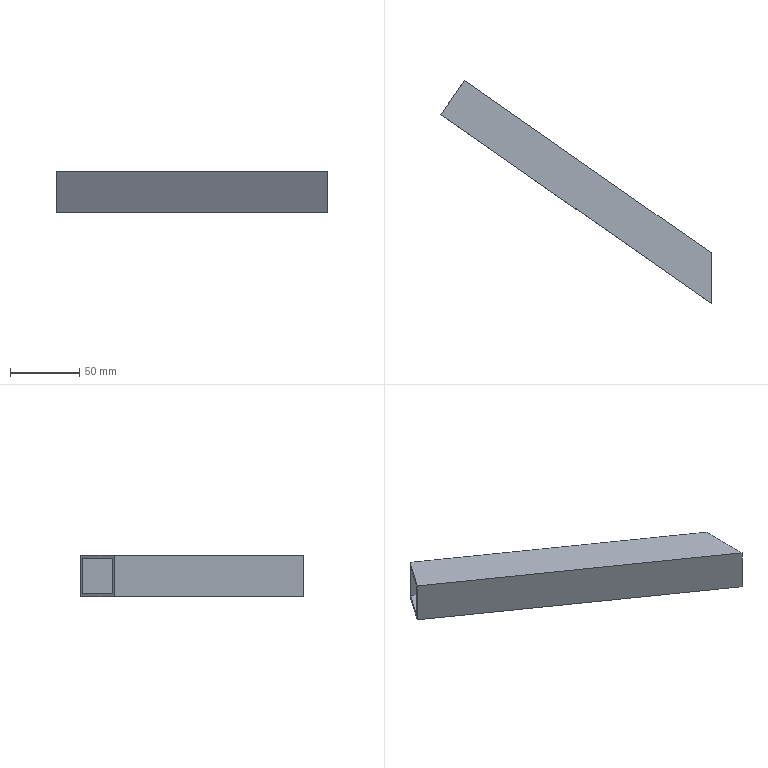Part | NX | features solid 2 | 1 solid | 10 faces | box 195.385 x 161.385 x 30 mm | volume 51076 mm3 | plane 10
STEP:
#1=CARTESIAN_POINT('',(-625.385,85.971,-40.));
#2=VERTEX_POINT('',#1);
#3=CARTESIAN_POINT('',(-608.178,110.546,-40.));
#4=VERTEX_POINT('',#3);
#5=CARTESIAN_POINT('',(-625.385,85.971,-40.));
#6=DIRECTION('',(-0.5736,-0.8192,0.));
#7=VECTOR('',#6,1000.);
#8=LINE('',#5,#7);
#9=EDGE_CURVE('',#2,#4,#8,.F.);
#10=ORIENTED_EDGE('',*,*,#9,.F.);
#11=CARTESIAN_POINT('',(-430.,-50.839,-40.));
#12=VERTEX_POINT('',#11);
#13=CARTESIAN_POINT('',(-543.47,28.614,-40.));
#14=DIRECTION('',(-0.8192,0.5736,0.));
#15=VECTOR('',#14,1000.);
#16=LINE('',#13,#15);
#17=EDGE_CURVE('',#2,#12,#16,.F.);
#18=ORIENTED_EDGE('',*,*,#17,.T.);
#19=CARTESIAN_POINT('',(-430.,-14.216,-40.));
#20=VERTEX_POINT('',#19);
#21=CARTESIAN_POINT('',(-430.,28.614,-40.));
#22=DIRECTION('',(0.,-1.,0.));
#23=VECTOR('',#22,1000.);
#24=LINE('',#21,#23);
#25=EDGE_CURVE('',#12,#20,#24,.F.);
#26=ORIENTED_EDGE('',*,*,#25,.T.);
#27=CARTESIAN_POINT('',(-526.263,53.188,-40.));
#28=DIRECTION('',(0.8192,-0.5736,0.));
#29=VECTOR('',#28,1000.);
#30=LINE('',#27,#29);
#31=EDGE_CURVE('',#4,#20,#30,.T.);
#32=ORIENTED_EDGE('',*,*,#31,.F.);
#33=EDGE_LOOP('',(#10,#18,#26,#32));
#34=FACE_BOUND('',#33,.T.);
#35=CARTESIAN_POINT('',(-543.47,28.614,-40.));
#36=DIRECTION('',(0.,0.,1.));
#37=DIRECTION('',(-0.8192,0.5736,0.));
#38=AXIS2_PLACEMENT_3D('',#35,#36,#37);
#39=PLANE('',#38);
#40=ADVANCED_FACE('',(#34),#39,.T.);
#41=CARTESIAN_POINT('',(-625.385,85.971,-70.));
#42=VERTEX_POINT('',#41);
#43=CARTESIAN_POINT('',(-430.,-50.839,-70.));
#44=VERTEX_POINT('',#43);
#45=CARTESIAN_POINT('',(-543.47,28.614,-70.));
#46=DIRECTION('',(0.8192,-0.5736,0.));
#47=VECTOR('',#46,1000.);
#48=LINE('',#45,#47);
#49=EDGE_CURVE('',#42,#44,#48,.T.);
#50=ORIENTED_EDGE('',*,*,#49,.F.);
#51=CARTESIAN_POINT('',(-608.178,110.546,-70.));
#52=VERTEX_POINT('',#51);
#53=CARTESIAN_POINT('',(-625.385,85.971,-70.));
#54=DIRECTION('',(-0.5736,-0.8192,0.));
#55=VECTOR('',#54,1000.);
#56=LINE('',#53,#55);
#57=EDGE_CURVE('',#42,#52,#56,.F.);
#58=ORIENTED_EDGE('',*,*,#57,.T.);
#59=CARTESIAN_POINT('',(-430.,-14.216,-70.));
#60=VERTEX_POINT('',#59);
#61=CARTESIAN_POINT('',(-526.263,53.188,-70.));
#62=DIRECTION('',(0.8192,-0.5736,0.));
#63=VECTOR('',#62,1000.);
#64=LINE('',#61,#63);
#65=EDGE_CURVE('',#52,#60,#64,.T.);
#66=ORIENTED_EDGE('',*,*,#65,.T.);
#67=CARTESIAN_POINT('',(-430.,-170.,-70.));
#68=DIRECTION('',(0.,1.,0.));
#69=VECTOR('',#68,1000.);
#70=LINE('',#67,#69);
#71=EDGE_CURVE('',#60,#44,#70,.F.);
#72=ORIENTED_EDGE('',*,*,#71,.T.);
#73=EDGE_LOOP('',(#50,#58,#66,#72));
#74=FACE_BOUND('',#73,.T.);
#75=CARTESIAN_POINT('',(-543.47,28.614,-70.));
#76=DIRECTION('',(0.,0.,1.));
#77=DIRECTION('',(-0.8192,0.5736,0.));
#78=AXIS2_PLACEMENT_3D('',#75,#76,#77);
#79=PLANE('',#78);
#80=ADVANCED_FACE('',(#74),#79,.F.);
#81=ORIENTED_EDGE('',*,*,#65,.F.);
#82=CARTESIAN_POINT('',(-608.178,110.546,-70.));
#83=DIRECTION('',(0.,0.,-1.));
#84=VECTOR('',#83,1000.);
#85=LINE('',#82,#84);
#86=EDGE_CURVE('',#52,#4,#85,.F.);
#87=ORIENTED_EDGE('',*,*,#86,.T.);
#88=ORIENTED_EDGE('',*,*,#31,.T.);
#89=CARTESIAN_POINT('',(-430.,-14.216,-95.));
#90=DIRECTION('',(0.,0.,1.));
#91=VECTOR('',#90,1000.);
#92=LINE('',#89,#91);
#93=EDGE_CURVE('',#20,#60,#92,.F.);
#94=ORIENTED_EDGE('',*,*,#93,.T.);
#95=EDGE_LOOP('',(#81,#87,#88,#94));
#96=FACE_BOUND('',#95,.T.);
#97=CARTESIAN_POINT('',(-526.263,53.188,-70.));
#98=DIRECTION('',(-0.5736,-0.8192,0.));
#99=DIRECTION('',(0.8192,-0.5736,0.));
#100=AXIS2_PLACEMENT_3D('',#97,#98,#99);
#101=PLANE('',#100);
#102=ADVANCED_FACE('',(#96),#101,.F.);
#103=ORIENTED_EDGE('',*,*,#17,.F.);
#104=CARTESIAN_POINT('',(-625.385,85.971,-70.));
#105=DIRECTION('',(0.,0.,-1.));
#106=VECTOR('',#105,1000.);
#107=LINE('',#104,#106);
#108=EDGE_CURVE('',#2,#42,#107,.T.);
#109=ORIENTED_EDGE('',*,*,#108,.T.);
#110=ORIENTED_EDGE('',*,*,#49,.T.);
#111=CARTESIAN_POINT('',(-430.,-50.839,-95.));
#112=DIRECTION('',(0.,0.,1.));
#113=VECTOR('',#112,1000.);
#114=LINE('',#111,#113);
#115=EDGE_CURVE('',#44,#12,#114,.T.);
#116=ORIENTED_EDGE('',*,*,#115,.T.);
#117=EDGE_LOOP('',(#103,#109,#110,#116));
#118=FACE_BOUND('',#117,.T.);
#119=CARTESIAN_POINT('',(-543.47,28.614,-70.));
#120=DIRECTION('',(-0.5736,-0.8192,0.));
#121=DIRECTION('',(0.8192,-0.5736,0.));
#122=AXIS2_PLACEMENT_3D('',#119,#120,#121);
#123=PLANE('',#122);
#124=ADVANCED_FACE('',(#118),#123,.T.);
#125=ORIENTED_EDGE('',*,*,#71,.F.);
#126=ORIENTED_EDGE('',*,*,#93,.F.);
#127=ORIENTED_EDGE('',*,*,#25,.F.);
#128=ORIENTED_EDGE('',*,*,#115,.F.);
#129=EDGE_LOOP('',(#125,#126,#127,#128));
#130=FACE_BOUND('',#129,.T.);
#131=CARTESIAN_POINT('',(-430.,-16.657,-42.));
#132=VERTEX_POINT('',#131);
#133=CARTESIAN_POINT('',(-430.,-16.657,-68.));
#134=VERTEX_POINT('',#133);
#135=CARTESIAN_POINT('',(-430.,-16.657,-95.));
#136=DIRECTION('',(0.,0.,1.));
#137=VECTOR('',#136,1000.);
#138=LINE('',#135,#137);
#139=EDGE_CURVE('',#132,#134,#138,.F.);
#140=ORIENTED_EDGE('',*,*,#139,.T.);
#141=CARTESIAN_POINT('',(-430.,-48.397,-68.));
#142=VERTEX_POINT('',#141);
#143=CARTESIAN_POINT('',(-430.,-170.,-68.));
#144=DIRECTION('',(0.,1.,0.));
#145=VECTOR('',#144,1000.);
#146=LINE('',#143,#145);
#147=EDGE_CURVE('',#134,#142,#146,.F.);
#148=ORIENTED_EDGE('',*,*,#147,.T.);
#149=CARTESIAN_POINT('',(-430.,-48.397,-42.));
#150=VERTEX_POINT('',#149);
#151=CARTESIAN_POINT('',(-430.,-48.397,-95.));
#152=DIRECTION('',(0.,0.,1.));
#153=VECTOR('',#152,1000.);
#154=LINE('',#151,#153);
#155=EDGE_CURVE('',#142,#150,#154,.T.);
#156=ORIENTED_EDGE('',*,*,#155,.T.);
#157=CARTESIAN_POINT('',(-430.,28.614,-42.));
#158=DIRECTION('',(0.,-1.,0.));
#159=VECTOR('',#158,1000.);
#160=LINE('',#157,#159);
#161=EDGE_CURVE('',#150,#132,#160,.F.);
#162=ORIENTED_EDGE('',*,*,#161,.T.);
#163=EDGE_LOOP('',(#140,#148,#156,#162));
#164=FACE_BOUND('',#163,.T.);
#165=CARTESIAN_POINT('',(-430.,-170.,-95.));
#166=DIRECTION('',(-1.,0.,0.));
#167=DIRECTION('',(0.,-1.,0.));
#168=AXIS2_PLACEMENT_3D('',#165,#166,#167);
#169=PLANE('',#168);
#170=ADVANCED_FACE('',(#130,#164),#169,.F.);
#171=CARTESIAN_POINT('',(-624.238,87.61,-42.));
#172=VERTEX_POINT('',#171);
#173=CARTESIAN_POINT('',(-542.323,30.252,-42.));
#174=DIRECTION('',(-0.8192,0.5736,0.));
#175=VECTOR('',#174,1000.);
#176=LINE('',#173,#175);
#177=EDGE_CURVE('',#172,#150,#176,.F.);
#178=ORIENTED_EDGE('',*,*,#177,.F.);
#179=CARTESIAN_POINT('',(-609.325,108.907,-42.));
#180=VERTEX_POINT('',#179);
#181=CARTESIAN_POINT('',(-625.385,85.971,-42.));
#182=DIRECTION('',(-0.5736,-0.8192,0.));
#183=VECTOR('',#182,1000.);
#184=LINE('',#181,#183);
#185=EDGE_CURVE('',#172,#180,#184,.F.);
#186=ORIENTED_EDGE('',*,*,#185,.T.);
#187=CARTESIAN_POINT('',(-527.41,51.55,-42.));
#188=DIRECTION('',(0.8192,-0.5736,0.));
#189=VECTOR('',#188,1000.);
#190=LINE('',#187,#189);
#191=EDGE_CURVE('',#180,#132,#190,.T.);
#192=ORIENTED_EDGE('',*,*,#191,.T.);
#193=ORIENTED_EDGE('',*,*,#161,.F.);
#194=EDGE_LOOP('',(#178,#186,#192,#193));
#195=FACE_BOUND('',#194,.T.);
#196=CARTESIAN_POINT('',(-543.47,28.614,-42.));
#197=DIRECTION('',(0.,0.,1.));
#198=DIRECTION('',(-0.8192,0.5736,0.));
#199=AXIS2_PLACEMENT_3D('',#196,#197,#198);
#200=PLANE('',#199);
#201=ADVANCED_FACE('',(#195),#200,.F.);
#202=CARTESIAN_POINT('',(-624.238,87.61,-68.));
#203=VERTEX_POINT('',#202);
#204=CARTESIAN_POINT('',(-609.325,108.907,-68.));
#205=VERTEX_POINT('',#204);
#206=CARTESIAN_POINT('',(-625.385,85.971,-68.));
#207=DIRECTION('',(-0.5736,-0.8192,0.));
#208=VECTOR('',#207,1000.);
#209=LINE('',#206,#208);
#210=EDGE_CURVE('',#203,#205,#209,.F.);
#211=ORIENTED_EDGE('',*,*,#210,.F.);
#212=CARTESIAN_POINT('',(-542.323,30.252,-68.));
#213=DIRECTION('',(-0.8192,0.5736,0.));
#214=VECTOR('',#213,1000.);
#215=LINE('',#212,#214);
#216=EDGE_CURVE('',#203,#142,#215,.F.);
#217=ORIENTED_EDGE('',*,*,#216,.T.);
#218=ORIENTED_EDGE('',*,*,#147,.F.);
#219=CARTESIAN_POINT('',(-527.41,51.55,-68.));
#220=DIRECTION('',(0.8192,-0.5736,0.));
#221=VECTOR('',#220,1000.);
#222=LINE('',#219,#221);
#223=EDGE_CURVE('',#205,#134,#222,.T.);
#224=ORIENTED_EDGE('',*,*,#223,.F.);
#225=EDGE_LOOP('',(#211,#217,#218,#224));
#226=FACE_BOUND('',#225,.T.);
#227=CARTESIAN_POINT('',(-543.47,28.614,-68.));
#228=DIRECTION('',(0.,0.,1.));
#229=DIRECTION('',(-0.8192,0.5736,0.));
#230=AXIS2_PLACEMENT_3D('',#227,#228,#229);
#231=PLANE('',#230);
#232=ADVANCED_FACE('',(#226),#231,.T.);
#233=CARTESIAN_POINT('',(-609.325,108.907,-70.));
#234=DIRECTION('',(0.,0.,-1.));
#235=VECTOR('',#234,1000.);
#236=LINE('',#233,#235);
#237=EDGE_CURVE('',#205,#180,#236,.F.);
#238=ORIENTED_EDGE('',*,*,#237,.F.);
#239=ORIENTED_EDGE('',*,*,#223,.T.);
#240=ORIENTED_EDGE('',*,*,#139,.F.);
#241=ORIENTED_EDGE('',*,*,#191,.F.);
#242=EDGE_LOOP('',(#238,#239,#240,#241));
#243=FACE_BOUND('',#242,.T.);
#244=CARTESIAN_POINT('',(-527.41,51.55,-70.));
#245=DIRECTION('',(-0.5736,-0.8192,0.));
#246=DIRECTION('',(0.8192,-0.5736,0.));
#247=AXIS2_PLACEMENT_3D('',#244,#245,#246);
#248=PLANE('',#247);
#249=ADVANCED_FACE('',(#243),#248,.T.);
#250=CARTESIAN_POINT('',(-624.238,87.61,-70.));
#251=DIRECTION('',(0.,0.,-1.));
#252=VECTOR('',#251,1000.);
#253=LINE('',#250,#252);
#254=EDGE_CURVE('',#172,#203,#253,.T.);
#255=ORIENTED_EDGE('',*,*,#254,.F.);
#256=ORIENTED_EDGE('',*,*,#177,.T.);
#257=ORIENTED_EDGE('',*,*,#155,.F.);
#258=ORIENTED_EDGE('',*,*,#216,.F.);
#259=EDGE_LOOP('',(#255,#256,#257,#258));
#260=FACE_BOUND('',#259,.T.);
#261=CARTESIAN_POINT('',(-542.323,30.252,-70.));
#262=DIRECTION('',(-0.5736,-0.8192,0.));
#263=DIRECTION('',(0.8192,-0.5736,0.));
#264=AXIS2_PLACEMENT_3D('',#261,#262,#263);
#265=PLANE('',#264);
#266=ADVANCED_FACE('',(#260),#265,.F.);
#267=ORIENTED_EDGE('',*,*,#9,.T.);
#268=ORIENTED_EDGE('',*,*,#86,.F.);
#269=ORIENTED_EDGE('',*,*,#57,.F.);
#270=ORIENTED_EDGE('',*,*,#108,.F.);
#271=EDGE_LOOP('',(#267,#268,#269,#270));
#272=FACE_BOUND('',#271,.T.);
#273=ORIENTED_EDGE('',*,*,#254,.T.);
#274=ORIENTED_EDGE('',*,*,#210,.T.);
#275=ORIENTED_EDGE('',*,*,#237,.T.);
#276=ORIENTED_EDGE('',*,*,#185,.F.);
#277=EDGE_LOOP('',(#273,#274,#275,#276));
#278=FACE_BOUND('',#277,.T.);
#279=CARTESIAN_POINT('',(-625.385,85.971,85.));
#280=DIRECTION('',(-0.8192,0.5736,0.));
#281=DIRECTION('',(-0.5736,-0.8192,0.));
#282=AXIS2_PLACEMENT_3D('',#279,#280,#281);
#283=PLANE('',#282);
#284=ADVANCED_FACE('',(#272,#278),#283,.T.);
#285=CLOSED_SHELL('',(#40,#80,#102,#124,#170,#201,#232,#249,#266,#284));
#286=MANIFOLD_SOLID_BREP('',#285);
#287=(LENGTH_UNIT()NAMED_UNIT(*)SI_UNIT(.MILLI.,.METRE.));
#288=UNCERTAINTY_MEASURE_WITH_UNIT(LENGTH_MEASURE(0.00001),#287,'','');
#289=(NAMED_UNIT(*)PLANE_ANGLE_UNIT()SI_UNIT($,.RADIAN.));
#290=(NAMED_UNIT(*)SI_UNIT($,.STERADIAN.)SOLID_ANGLE_UNIT());
#291=(GEOMETRIC_REPRESENTATION_CONTEXT(3)GLOBAL_UNCERTAINTY_ASSIGNED_CONTEXT((#288))GLOBAL_UNIT_ASSIGNED_CONTEXT((#287,#289,#290))REPRESENTATION_CONTEXT('',''));
#292=ADVANCED_BREP_SHAPE_REPRESENTATION('',(#286),#291);